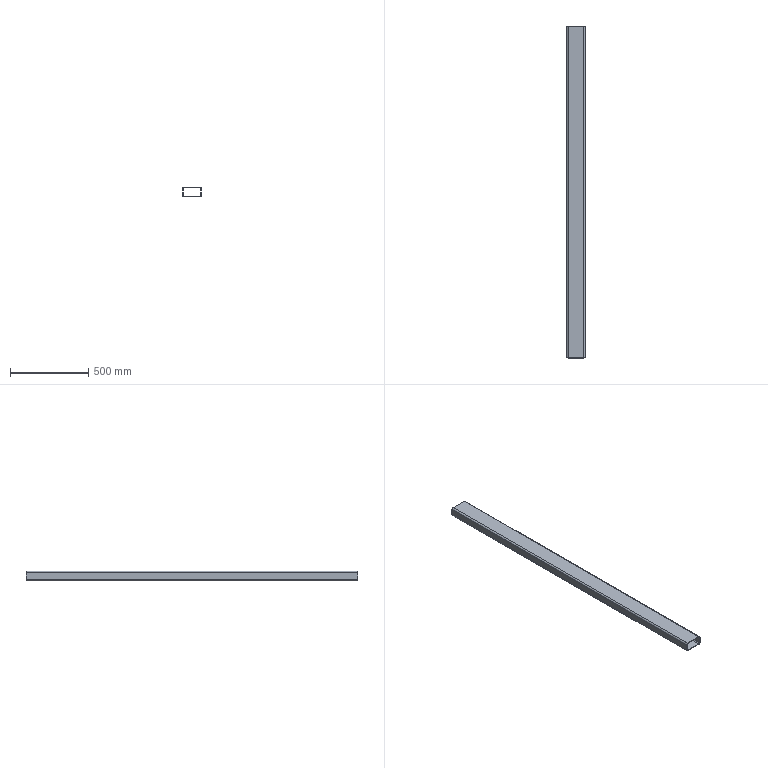Part | SolidWorks | features ExtruThin 1 | 1 solid | 18 faces | box 120 x 2124 x 60 mm | volume 2805936 mm3 | plane 10 | cylinder 8 | commonest cylinder face diameters 12 x4 20 x4
STEP:
#1=CARTESIAN_POINT('',(60.,1062.,-20.));
#2=VERTEX_POINT('',#1);
#3=CARTESIAN_POINT('',(50.,1062.,-30.));
#4=VERTEX_POINT('',#3);
#5=CARTESIAN_POINT('',(50.,1062.,-20.));
#6=DIRECTION('',(0.,1.,0.));
#7=DIRECTION('',(0.,0.,-1.));
#8=AXIS2_PLACEMENT_3D('',#5,#6,#7);
#9=CIRCLE('',#8,10.);
#10=EDGE_CURVE('',#2,#4,#9,.T.);
#11=ORIENTED_EDGE('',*,*,#10,.T.);
#12=CARTESIAN_POINT('',(-50.,1062.,-30.));
#13=VERTEX_POINT('',#12);
#14=CARTESIAN_POINT('',(-50.,1062.,-30.));
#15=DIRECTION('',(-1.,0.,0.));
#16=VECTOR('',#15,1000.);
#17=LINE('',#14,#16);
#18=EDGE_CURVE('',#4,#13,#17,.T.);
#19=ORIENTED_EDGE('',*,*,#18,.T.);
#20=CARTESIAN_POINT('',(-60.,1062.,-20.));
#21=VERTEX_POINT('',#20);
#22=CARTESIAN_POINT('',(-50.,1062.,-20.));
#23=DIRECTION('',(0.,1.,0.));
#24=DIRECTION('',(0.,0.,1.));
#25=AXIS2_PLACEMENT_3D('',#22,#23,#24);
#26=CIRCLE('',#25,10.);
#27=EDGE_CURVE('',#13,#21,#26,.T.);
#28=ORIENTED_EDGE('',*,*,#27,.T.);
#29=CARTESIAN_POINT('',(-60.,1062.,20.));
#30=VERTEX_POINT('',#29);
#31=CARTESIAN_POINT('',(-60.,1062.,-20.));
#32=DIRECTION('',(0.,0.,1.));
#33=VECTOR('',#32,1000.);
#34=LINE('',#31,#33);
#35=EDGE_CURVE('',#21,#30,#34,.T.);
#36=ORIENTED_EDGE('',*,*,#35,.T.);
#37=CARTESIAN_POINT('',(-50.,1062.,30.));
#38=VERTEX_POINT('',#37);
#39=CARTESIAN_POINT('',(-50.,1062.,20.));
#40=DIRECTION('',(0.,1.,0.));
#41=DIRECTION('',(0.,0.,1.));
#42=AXIS2_PLACEMENT_3D('',#39,#40,#41);
#43=CIRCLE('',#42,10.);
#44=EDGE_CURVE('',#30,#38,#43,.T.);
#45=ORIENTED_EDGE('',*,*,#44,.T.);
#46=CARTESIAN_POINT('',(50.,1062.,30.));
#47=VERTEX_POINT('',#46);
#48=CARTESIAN_POINT('',(-50.,1062.,30.));
#49=DIRECTION('',(1.,0.,0.));
#50=VECTOR('',#49,1000.);
#51=LINE('',#48,#50);
#52=EDGE_CURVE('',#38,#47,#51,.T.);
#53=ORIENTED_EDGE('',*,*,#52,.T.);
#54=CARTESIAN_POINT('',(60.,1062.,20.));
#55=VERTEX_POINT('',#54);
#56=CARTESIAN_POINT('',(50.,1062.,20.));
#57=DIRECTION('',(0.,1.,0.));
#58=DIRECTION('',(0.,0.,1.));
#59=AXIS2_PLACEMENT_3D('',#56,#57,#58);
#60=CIRCLE('',#59,10.);
#61=EDGE_CURVE('',#47,#55,#60,.T.);
#62=ORIENTED_EDGE('',*,*,#61,.T.);
#63=CARTESIAN_POINT('',(60.,1062.,-20.));
#64=DIRECTION('',(0.,0.,-1.));
#65=VECTOR('',#64,1000.);
#66=LINE('',#63,#65);
#67=EDGE_CURVE('',#55,#2,#66,.T.);
#68=ORIENTED_EDGE('',*,*,#67,.T.);
#69=EDGE_LOOP('',(#11,#19,#28,#36,#45,#53,#62,#68));
#70=FACE_OUTER_BOUND('',#69,.T.);
#71=CARTESIAN_POINT('',(50.,1062.,-26.));
#72=VERTEX_POINT('',#71);
#73=CARTESIAN_POINT('',(-50.,1062.,-26.));
#74=VERTEX_POINT('',#73);
#75=CARTESIAN_POINT('',(50.,1062.,-26.));
#76=DIRECTION('',(-1.,0.,0.));
#77=VECTOR('',#76,1000.);
#78=LINE('',#75,#77);
#79=EDGE_CURVE('',#72,#74,#78,.T.);
#80=ORIENTED_EDGE('',*,*,#79,.F.);
#81=CARTESIAN_POINT('',(56.,1062.,-20.));
#82=VERTEX_POINT('',#81);
#83=CARTESIAN_POINT('',(50.,1062.,-20.));
#84=DIRECTION('',(0.,1.,0.));
#85=DIRECTION('',(-1.,0.,0.));
#86=AXIS2_PLACEMENT_3D('',#83,#84,#85);
#87=CIRCLE('',#86,6.);
#88=EDGE_CURVE('',#82,#72,#87,.T.);
#89=ORIENTED_EDGE('',*,*,#88,.F.);
#90=CARTESIAN_POINT('',(56.,1062.,20.));
#91=VERTEX_POINT('',#90);
#92=CARTESIAN_POINT('',(56.,1062.,-20.));
#93=DIRECTION('',(0.,0.,-1.));
#94=VECTOR('',#93,1000.);
#95=LINE('',#92,#94);
#96=EDGE_CURVE('',#91,#82,#95,.T.);
#97=ORIENTED_EDGE('',*,*,#96,.F.);
#98=CARTESIAN_POINT('',(50.,1062.,26.));
#99=VERTEX_POINT('',#98);
#100=CARTESIAN_POINT('',(50.,1062.,20.));
#101=DIRECTION('',(0.,1.,0.));
#102=DIRECTION('',(-1.,0.,0.));
#103=AXIS2_PLACEMENT_3D('',#100,#101,#102);
#104=CIRCLE('',#103,6.);
#105=EDGE_CURVE('',#99,#91,#104,.T.);
#106=ORIENTED_EDGE('',*,*,#105,.F.);
#107=CARTESIAN_POINT('',(-50.,1062.,26.));
#108=VERTEX_POINT('',#107);
#109=CARTESIAN_POINT('',(50.,1062.,26.));
#110=DIRECTION('',(1.,0.,0.));
#111=VECTOR('',#110,1000.);
#112=LINE('',#109,#111);
#113=EDGE_CURVE('',#108,#99,#112,.T.);
#114=ORIENTED_EDGE('',*,*,#113,.F.);
#115=CARTESIAN_POINT('',(-56.,1062.,20.));
#116=VERTEX_POINT('',#115);
#117=CARTESIAN_POINT('',(-50.,1062.,20.));
#118=DIRECTION('',(0.,1.,0.));
#119=DIRECTION('',(-1.,0.,0.));
#120=AXIS2_PLACEMENT_3D('',#117,#118,#119);
#121=CIRCLE('',#120,6.);
#122=EDGE_CURVE('',#116,#108,#121,.T.);
#123=ORIENTED_EDGE('',*,*,#122,.F.);
#124=CARTESIAN_POINT('',(-56.,1062.,-20.));
#125=VERTEX_POINT('',#124);
#126=CARTESIAN_POINT('',(-56.,1062.,-20.));
#127=DIRECTION('',(0.,0.,1.));
#128=VECTOR('',#127,1000.);
#129=LINE('',#126,#128);
#130=EDGE_CURVE('',#125,#116,#129,.T.);
#131=ORIENTED_EDGE('',*,*,#130,.F.);
#132=CARTESIAN_POINT('',(-50.,1062.,-20.));
#133=DIRECTION('',(0.,1.,0.));
#134=DIRECTION('',(-1.,0.,0.));
#135=AXIS2_PLACEMENT_3D('',#132,#133,#134);
#136=CIRCLE('',#135,6.);
#137=EDGE_CURVE('',#74,#125,#136,.T.);
#138=ORIENTED_EDGE('',*,*,#137,.F.);
#139=EDGE_LOOP('',(#80,#89,#97,#106,#114,#123,#131,#138));
#140=FACE_BOUND('',#139,.T.);
#141=CARTESIAN_POINT('',(50.,1062.,-20.));
#142=DIRECTION('',(0.,1.,0.));
#143=DIRECTION('',(0.,0.,1.));
#144=AXIS2_PLACEMENT_3D('',#141,#142,#143);
#145=PLANE('',#144);
#146=ADVANCED_FACE('',(#70,#140),#145,.T.);
#147=CARTESIAN_POINT('',(60.,-1062.,-20.));
#148=VERTEX_POINT('',#147);
#149=CARTESIAN_POINT('',(50.,-1062.,-30.));
#150=VERTEX_POINT('',#149);
#151=CARTESIAN_POINT('',(50.,-1062.,-20.));
#152=DIRECTION('',(0.,1.,0.));
#153=DIRECTION('',(0.,0.,-1.));
#154=AXIS2_PLACEMENT_3D('',#151,#152,#153);
#155=CIRCLE('',#154,10.);
#156=EDGE_CURVE('',#148,#150,#155,.T.);
#157=ORIENTED_EDGE('',*,*,#156,.F.);
#158=CARTESIAN_POINT('',(60.,-1062.,20.));
#159=VERTEX_POINT('',#158);
#160=CARTESIAN_POINT('',(60.,-1062.,-20.));
#161=DIRECTION('',(0.,0.,-1.));
#162=VECTOR('',#161,1000.);
#163=LINE('',#160,#162);
#164=EDGE_CURVE('',#159,#148,#163,.T.);
#165=ORIENTED_EDGE('',*,*,#164,.F.);
#166=CARTESIAN_POINT('',(50.,-1062.,30.));
#167=VERTEX_POINT('',#166);
#168=CARTESIAN_POINT('',(50.,-1062.,20.));
#169=DIRECTION('',(0.,1.,0.));
#170=DIRECTION('',(0.,0.,1.));
#171=AXIS2_PLACEMENT_3D('',#168,#169,#170);
#172=CIRCLE('',#171,10.);
#173=EDGE_CURVE('',#167,#159,#172,.T.);
#174=ORIENTED_EDGE('',*,*,#173,.F.);
#175=CARTESIAN_POINT('',(-50.,-1062.,30.));
#176=VERTEX_POINT('',#175);
#177=CARTESIAN_POINT('',(-50.,-1062.,30.));
#178=DIRECTION('',(1.,0.,0.));
#179=VECTOR('',#178,1000.);
#180=LINE('',#177,#179);
#181=EDGE_CURVE('',#176,#167,#180,.T.);
#182=ORIENTED_EDGE('',*,*,#181,.F.);
#183=CARTESIAN_POINT('',(-60.,-1062.,20.));
#184=VERTEX_POINT('',#183);
#185=CARTESIAN_POINT('',(-50.,-1062.,20.));
#186=DIRECTION('',(0.,1.,0.));
#187=DIRECTION('',(0.,0.,1.));
#188=AXIS2_PLACEMENT_3D('',#185,#186,#187);
#189=CIRCLE('',#188,10.);
#190=EDGE_CURVE('',#184,#176,#189,.T.);
#191=ORIENTED_EDGE('',*,*,#190,.F.);
#192=CARTESIAN_POINT('',(-60.,-1062.,-20.));
#193=VERTEX_POINT('',#192);
#194=CARTESIAN_POINT('',(-60.,-1062.,-20.));
#195=DIRECTION('',(0.,0.,1.));
#196=VECTOR('',#195,1000.);
#197=LINE('',#194,#196);
#198=EDGE_CURVE('',#193,#184,#197,.T.);
#199=ORIENTED_EDGE('',*,*,#198,.F.);
#200=CARTESIAN_POINT('',(-50.,-1062.,-30.));
#201=VERTEX_POINT('',#200);
#202=CARTESIAN_POINT('',(-50.,-1062.,-20.));
#203=DIRECTION('',(0.,1.,0.));
#204=DIRECTION('',(0.,0.,1.));
#205=AXIS2_PLACEMENT_3D('',#202,#203,#204);
#206=CIRCLE('',#205,10.);
#207=EDGE_CURVE('',#201,#193,#206,.T.);
#208=ORIENTED_EDGE('',*,*,#207,.F.);
#209=CARTESIAN_POINT('',(-50.,-1062.,-30.));
#210=DIRECTION('',(-1.,0.,0.));
#211=VECTOR('',#210,1000.);
#212=LINE('',#209,#211);
#213=EDGE_CURVE('',#150,#201,#212,.T.);
#214=ORIENTED_EDGE('',*,*,#213,.F.);
#215=EDGE_LOOP('',(#157,#165,#174,#182,#191,#199,#208,#214));
#216=FACE_OUTER_BOUND('',#215,.T.);
#217=CARTESIAN_POINT('',(56.,-1062.,-20.));
#218=VERTEX_POINT('',#217);
#219=CARTESIAN_POINT('',(50.,-1062.,-26.));
#220=VERTEX_POINT('',#219);
#221=CARTESIAN_POINT('',(50.,-1062.,-20.));
#222=DIRECTION('',(0.,1.,0.));
#223=DIRECTION('',(-1.,0.,0.));
#224=AXIS2_PLACEMENT_3D('',#221,#222,#223);
#225=CIRCLE('',#224,6.);
#226=EDGE_CURVE('',#218,#220,#225,.T.);
#227=ORIENTED_EDGE('',*,*,#226,.T.);
#228=CARTESIAN_POINT('',(-50.,-1062.,-26.));
#229=VERTEX_POINT('',#228);
#230=CARTESIAN_POINT('',(50.,-1062.,-26.));
#231=DIRECTION('',(-1.,0.,0.));
#232=VECTOR('',#231,1000.);
#233=LINE('',#230,#232);
#234=EDGE_CURVE('',#220,#229,#233,.T.);
#235=ORIENTED_EDGE('',*,*,#234,.T.);
#236=CARTESIAN_POINT('',(-56.,-1062.,-20.));
#237=VERTEX_POINT('',#236);
#238=CARTESIAN_POINT('',(-50.,-1062.,-20.));
#239=DIRECTION('',(0.,1.,0.));
#240=DIRECTION('',(-1.,0.,0.));
#241=AXIS2_PLACEMENT_3D('',#238,#239,#240);
#242=CIRCLE('',#241,6.);
#243=EDGE_CURVE('',#229,#237,#242,.T.);
#244=ORIENTED_EDGE('',*,*,#243,.T.);
#245=CARTESIAN_POINT('',(-56.,-1062.,20.));
#246=VERTEX_POINT('',#245);
#247=CARTESIAN_POINT('',(-56.,-1062.,-20.));
#248=DIRECTION('',(0.,0.,1.));
#249=VECTOR('',#248,1000.);
#250=LINE('',#247,#249);
#251=EDGE_CURVE('',#237,#246,#250,.T.);
#252=ORIENTED_EDGE('',*,*,#251,.T.);
#253=CARTESIAN_POINT('',(-50.,-1062.,26.));
#254=VERTEX_POINT('',#253);
#255=CARTESIAN_POINT('',(-50.,-1062.,20.));
#256=DIRECTION('',(0.,1.,0.));
#257=DIRECTION('',(-1.,0.,0.));
#258=AXIS2_PLACEMENT_3D('',#255,#256,#257);
#259=CIRCLE('',#258,6.);
#260=EDGE_CURVE('',#246,#254,#259,.T.);
#261=ORIENTED_EDGE('',*,*,#260,.T.);
#262=CARTESIAN_POINT('',(50.,-1062.,26.));
#263=VERTEX_POINT('',#262);
#264=CARTESIAN_POINT('',(50.,-1062.,26.));
#265=DIRECTION('',(1.,0.,0.));
#266=VECTOR('',#265,1000.);
#267=LINE('',#264,#266);
#268=EDGE_CURVE('',#254,#263,#267,.T.);
#269=ORIENTED_EDGE('',*,*,#268,.T.);
#270=CARTESIAN_POINT('',(56.,-1062.,20.));
#271=VERTEX_POINT('',#270);
#272=CARTESIAN_POINT('',(50.,-1062.,20.));
#273=DIRECTION('',(0.,1.,0.));
#274=DIRECTION('',(-1.,0.,0.));
#275=AXIS2_PLACEMENT_3D('',#272,#273,#274);
#276=CIRCLE('',#275,6.);
#277=EDGE_CURVE('',#263,#271,#276,.T.);
#278=ORIENTED_EDGE('',*,*,#277,.T.);
#279=CARTESIAN_POINT('',(56.,-1062.,-20.));
#280=DIRECTION('',(0.,0.,-1.));
#281=VECTOR('',#280,1000.);
#282=LINE('',#279,#281);
#283=EDGE_CURVE('',#271,#218,#282,.T.);
#284=ORIENTED_EDGE('',*,*,#283,.T.);
#285=EDGE_LOOP('',(#227,#235,#244,#252,#261,#269,#278,#284));
#286=FACE_BOUND('',#285,.T.);
#287=CARTESIAN_POINT('',(50.,-1062.,-20.));
#288=DIRECTION('',(0.,1.,0.));
#289=DIRECTION('',(0.,0.,1.));
#290=AXIS2_PLACEMENT_3D('',#287,#288,#289);
#291=PLANE('',#290);
#292=ADVANCED_FACE('',(#216,#286),#291,.F.);
#293=ORIENTED_EDGE('',*,*,#156,.T.);
#294=CARTESIAN_POINT('',(50.,1062.,-30.));
#295=DIRECTION('',(0.,-1.,0.));
#296=VECTOR('',#295,1000.);
#297=LINE('',#294,#296);
#298=EDGE_CURVE('',#4,#150,#297,.T.);
#299=ORIENTED_EDGE('',*,*,#298,.F.);
#300=ORIENTED_EDGE('',*,*,#10,.F.);
#301=CARTESIAN_POINT('',(60.,1062.,-20.));
#302=DIRECTION('',(0.,-1.,0.));
#303=VECTOR('',#302,1000.);
#304=LINE('',#301,#303);
#305=EDGE_CURVE('',#2,#148,#304,.T.);
#306=ORIENTED_EDGE('',*,*,#305,.T.);
#307=EDGE_LOOP('',(#293,#299,#300,#306));
#308=FACE_OUTER_BOUND('',#307,.T.);
#309=CARTESIAN_POINT('',(50.,1062.,-20.));
#310=DIRECTION('',(0.,-1.,0.));
#311=DIRECTION('',(0.,0.,-1.));
#312=AXIS2_PLACEMENT_3D('',#309,#310,#311);
#313=CYLINDRICAL_SURFACE('',#312,10.);
#314=ADVANCED_FACE('',(#308),#313,.T.);
#315=ORIENTED_EDGE('',*,*,#213,.T.);
#316=CARTESIAN_POINT('',(-50.,1062.,-30.));
#317=DIRECTION('',(0.,-1.,0.));
#318=VECTOR('',#317,1000.);
#319=LINE('',#316,#318);
#320=EDGE_CURVE('',#13,#201,#319,.T.);
#321=ORIENTED_EDGE('',*,*,#320,.F.);
#322=ORIENTED_EDGE('',*,*,#18,.F.);
#323=ORIENTED_EDGE('',*,*,#298,.T.);
#324=EDGE_LOOP('',(#315,#321,#322,#323));
#325=FACE_OUTER_BOUND('',#324,.T.);
#326=CARTESIAN_POINT('',(-50.,1062.,-30.));
#327=DIRECTION('',(0.,0.,1.));
#328=DIRECTION('',(1.,0.,0.));
#329=AXIS2_PLACEMENT_3D('',#326,#327,#328);
#330=PLANE('',#329);
#331=ADVANCED_FACE('',(#325),#330,.F.);
#332=ORIENTED_EDGE('',*,*,#207,.T.);
#333=CARTESIAN_POINT('',(-60.,1062.,-20.));
#334=DIRECTION('',(0.,-1.,0.));
#335=VECTOR('',#334,1000.);
#336=LINE('',#333,#335);
#337=EDGE_CURVE('',#21,#193,#336,.T.);
#338=ORIENTED_EDGE('',*,*,#337,.F.);
#339=ORIENTED_EDGE('',*,*,#27,.F.);
#340=ORIENTED_EDGE('',*,*,#320,.T.);
#341=EDGE_LOOP('',(#332,#338,#339,#340));
#342=FACE_OUTER_BOUND('',#341,.T.);
#343=CARTESIAN_POINT('',(-50.,1062.,-20.));
#344=DIRECTION('',(0.,-1.,0.));
#345=DIRECTION('',(0.,0.,-1.));
#346=AXIS2_PLACEMENT_3D('',#343,#344,#345);
#347=CYLINDRICAL_SURFACE('',#346,10.);
#348=ADVANCED_FACE('',(#342),#347,.T.);
#349=ORIENTED_EDGE('',*,*,#198,.T.);
#350=CARTESIAN_POINT('',(-60.,1062.,20.));
#351=DIRECTION('',(0.,-1.,0.));
#352=VECTOR('',#351,1000.);
#353=LINE('',#350,#352);
#354=EDGE_CURVE('',#30,#184,#353,.T.);
#355=ORIENTED_EDGE('',*,*,#354,.F.);
#356=ORIENTED_EDGE('',*,*,#35,.F.);
#357=ORIENTED_EDGE('',*,*,#337,.T.);
#358=EDGE_LOOP('',(#349,#355,#356,#357));
#359=FACE_OUTER_BOUND('',#358,.T.);
#360=CARTESIAN_POINT('',(-60.,1062.,-20.));
#361=DIRECTION('',(1.,0.,0.));
#362=DIRECTION('',(0.,0.,-1.));
#363=AXIS2_PLACEMENT_3D('',#360,#361,#362);
#364=PLANE('',#363);
#365=ADVANCED_FACE('',(#359),#364,.F.);
#366=ORIENTED_EDGE('',*,*,#190,.T.);
#367=CARTESIAN_POINT('',(-50.,1062.,30.));
#368=DIRECTION('',(0.,-1.,0.));
#369=VECTOR('',#368,1000.);
#370=LINE('',#367,#369);
#371=EDGE_CURVE('',#38,#176,#370,.T.);
#372=ORIENTED_EDGE('',*,*,#371,.F.);
#373=ORIENTED_EDGE('',*,*,#44,.F.);
#374=ORIENTED_EDGE('',*,*,#354,.T.);
#375=EDGE_LOOP('',(#366,#372,#373,#374));
#376=FACE_OUTER_BOUND('',#375,.T.);
#377=CARTESIAN_POINT('',(-50.,1062.,20.));
#378=DIRECTION('',(0.,-1.,0.));
#379=DIRECTION('',(0.,0.,-1.));
#380=AXIS2_PLACEMENT_3D('',#377,#378,#379);
#381=CYLINDRICAL_SURFACE('',#380,10.);
#382=ADVANCED_FACE('',(#376),#381,.T.);
#383=ORIENTED_EDGE('',*,*,#181,.T.);
#384=CARTESIAN_POINT('',(50.,1062.,30.));
#385=DIRECTION('',(0.,-1.,0.));
#386=VECTOR('',#385,1000.);
#387=LINE('',#384,#386);
#388=EDGE_CURVE('',#47,#167,#387,.T.);
#389=ORIENTED_EDGE('',*,*,#388,.F.);
#390=ORIENTED_EDGE('',*,*,#52,.F.);
#391=ORIENTED_EDGE('',*,*,#371,.T.);
#392=EDGE_LOOP('',(#383,#389,#390,#391));
#393=FACE_OUTER_BOUND('',#392,.T.);
#394=CARTESIAN_POINT('',(-50.,1062.,30.));
#395=DIRECTION('',(0.,0.,-1.));
#396=DIRECTION('',(-1.,0.,0.));
#397=AXIS2_PLACEMENT_3D('',#394,#395,#396);
#398=PLANE('',#397);
#399=ADVANCED_FACE('',(#393),#398,.F.);
#400=ORIENTED_EDGE('',*,*,#173,.T.);
#401=CARTESIAN_POINT('',(60.,1062.,20.));
#402=DIRECTION('',(0.,-1.,0.));
#403=VECTOR('',#402,1000.);
#404=LINE('',#401,#403);
#405=EDGE_CURVE('',#55,#159,#404,.T.);
#406=ORIENTED_EDGE('',*,*,#405,.F.);
#407=ORIENTED_EDGE('',*,*,#61,.F.);
#408=ORIENTED_EDGE('',*,*,#388,.T.);
#409=EDGE_LOOP('',(#400,#406,#407,#408));
#410=FACE_OUTER_BOUND('',#409,.T.);
#411=CARTESIAN_POINT('',(50.,1062.,20.));
#412=DIRECTION('',(0.,-1.,0.));
#413=DIRECTION('',(0.,0.,-1.));
#414=AXIS2_PLACEMENT_3D('',#411,#412,#413);
#415=CYLINDRICAL_SURFACE('',#414,10.);
#416=ADVANCED_FACE('',(#410),#415,.T.);
#417=ORIENTED_EDGE('',*,*,#164,.T.);
#418=ORIENTED_EDGE('',*,*,#305,.F.);
#419=ORIENTED_EDGE('',*,*,#67,.F.);
#420=ORIENTED_EDGE('',*,*,#405,.T.);
#421=EDGE_LOOP('',(#417,#418,#419,#420));
#422=FACE_OUTER_BOUND('',#421,.T.);
#423=CARTESIAN_POINT('',(60.,1062.,-20.));
#424=DIRECTION('',(-1.,0.,0.));
#425=DIRECTION('',(0.,0.,1.));
#426=AXIS2_PLACEMENT_3D('',#423,#424,#425);
#427=PLANE('',#426);
#428=ADVANCED_FACE('',(#422),#427,.F.);
#429=ORIENTED_EDGE('',*,*,#226,.F.);
#430=CARTESIAN_POINT('',(56.,1062.,-20.));
#431=DIRECTION('',(0.,-1.,0.));
#432=VECTOR('',#431,1000.);
#433=LINE('',#430,#432);
#434=EDGE_CURVE('',#82,#218,#433,.T.);
#435=ORIENTED_EDGE('',*,*,#434,.F.);
#436=ORIENTED_EDGE('',*,*,#88,.T.);
#437=CARTESIAN_POINT('',(50.,1062.,-26.));
#438=DIRECTION('',(0.,-1.,0.));
#439=VECTOR('',#438,1000.);
#440=LINE('',#437,#439);
#441=EDGE_CURVE('',#72,#220,#440,.T.);
#442=ORIENTED_EDGE('',*,*,#441,.T.);
#443=EDGE_LOOP('',(#429,#435,#436,#442));
#444=FACE_OUTER_BOUND('',#443,.T.);
#445=CARTESIAN_POINT('',(50.,1062.,-20.));
#446=DIRECTION('',(0.,-1.,0.));
#447=DIRECTION('',(0.,0.,-1.));
#448=AXIS2_PLACEMENT_3D('',#445,#446,#447);
#449=CYLINDRICAL_SURFACE('',#448,6.);
#450=ADVANCED_FACE('',(#444),#449,.F.);
#451=ORIENTED_EDGE('',*,*,#234,.F.);
#452=ORIENTED_EDGE('',*,*,#441,.F.);
#453=ORIENTED_EDGE('',*,*,#79,.T.);
#454=CARTESIAN_POINT('',(-50.,1062.,-26.));
#455=DIRECTION('',(0.,-1.,0.));
#456=VECTOR('',#455,1000.);
#457=LINE('',#454,#456);
#458=EDGE_CURVE('',#74,#229,#457,.T.);
#459=ORIENTED_EDGE('',*,*,#458,.T.);
#460=EDGE_LOOP('',(#451,#452,#453,#459));
#461=FACE_OUTER_BOUND('',#460,.T.);
#462=CARTESIAN_POINT('',(50.,1062.,-26.));
#463=DIRECTION('',(0.,0.,1.));
#464=DIRECTION('',(1.,0.,0.));
#465=AXIS2_PLACEMENT_3D('',#462,#463,#464);
#466=PLANE('',#465);
#467=ADVANCED_FACE('',(#461),#466,.T.);
#468=ORIENTED_EDGE('',*,*,#243,.F.);
#469=ORIENTED_EDGE('',*,*,#458,.F.);
#470=ORIENTED_EDGE('',*,*,#137,.T.);
#471=CARTESIAN_POINT('',(-56.,1062.,-20.));
#472=DIRECTION('',(0.,-1.,0.));
#473=VECTOR('',#472,1000.);
#474=LINE('',#471,#473);
#475=EDGE_CURVE('',#125,#237,#474,.T.);
#476=ORIENTED_EDGE('',*,*,#475,.T.);
#477=EDGE_LOOP('',(#468,#469,#470,#476));
#478=FACE_OUTER_BOUND('',#477,.T.);
#479=CARTESIAN_POINT('',(-50.,1062.,-20.));
#480=DIRECTION('',(0.,-1.,0.));
#481=DIRECTION('',(0.,0.,-1.));
#482=AXIS2_PLACEMENT_3D('',#479,#480,#481);
#483=CYLINDRICAL_SURFACE('',#482,6.);
#484=ADVANCED_FACE('',(#478),#483,.F.);
#485=ORIENTED_EDGE('',*,*,#251,.F.);
#486=ORIENTED_EDGE('',*,*,#475,.F.);
#487=ORIENTED_EDGE('',*,*,#130,.T.);
#488=CARTESIAN_POINT('',(-56.,1062.,20.));
#489=DIRECTION('',(0.,-1.,0.));
#490=VECTOR('',#489,1000.);
#491=LINE('',#488,#490);
#492=EDGE_CURVE('',#116,#246,#491,.T.);
#493=ORIENTED_EDGE('',*,*,#492,.T.);
#494=EDGE_LOOP('',(#485,#486,#487,#493));
#495=FACE_OUTER_BOUND('',#494,.T.);
#496=CARTESIAN_POINT('',(-56.,1062.,-20.));
#497=DIRECTION('',(1.,0.,0.));
#498=DIRECTION('',(0.,0.,-1.));
#499=AXIS2_PLACEMENT_3D('',#496,#497,#498);
#500=PLANE('',#499);
#501=ADVANCED_FACE('',(#495),#500,.T.);
#502=ORIENTED_EDGE('',*,*,#260,.F.);
#503=ORIENTED_EDGE('',*,*,#492,.F.);
#504=ORIENTED_EDGE('',*,*,#122,.T.);
#505=CARTESIAN_POINT('',(-50.,1062.,26.));
#506=DIRECTION('',(0.,-1.,0.));
#507=VECTOR('',#506,1000.);
#508=LINE('',#505,#507);
#509=EDGE_CURVE('',#108,#254,#508,.T.);
#510=ORIENTED_EDGE('',*,*,#509,.T.);
#511=EDGE_LOOP('',(#502,#503,#504,#510));
#512=FACE_OUTER_BOUND('',#511,.T.);
#513=CARTESIAN_POINT('',(-50.,1062.,20.));
#514=DIRECTION('',(0.,-1.,0.));
#515=DIRECTION('',(0.,0.,-1.));
#516=AXIS2_PLACEMENT_3D('',#513,#514,#515);
#517=CYLINDRICAL_SURFACE('',#516,6.);
#518=ADVANCED_FACE('',(#512),#517,.F.);
#519=ORIENTED_EDGE('',*,*,#268,.F.);
#520=ORIENTED_EDGE('',*,*,#509,.F.);
#521=ORIENTED_EDGE('',*,*,#113,.T.);
#522=CARTESIAN_POINT('',(50.,1062.,26.));
#523=DIRECTION('',(0.,-1.,0.));
#524=VECTOR('',#523,1000.);
#525=LINE('',#522,#524);
#526=EDGE_CURVE('',#99,#263,#525,.T.);
#527=ORIENTED_EDGE('',*,*,#526,.T.);
#528=EDGE_LOOP('',(#519,#520,#521,#527));
#529=FACE_OUTER_BOUND('',#528,.T.);
#530=CARTESIAN_POINT('',(50.,1062.,26.));
#531=DIRECTION('',(0.,0.,-1.));
#532=DIRECTION('',(-1.,0.,0.));
#533=AXIS2_PLACEMENT_3D('',#530,#531,#532);
#534=PLANE('',#533);
#535=ADVANCED_FACE('',(#529),#534,.T.);
#536=ORIENTED_EDGE('',*,*,#277,.F.);
#537=ORIENTED_EDGE('',*,*,#526,.F.);
#538=ORIENTED_EDGE('',*,*,#105,.T.);
#539=CARTESIAN_POINT('',(56.,1062.,20.));
#540=DIRECTION('',(0.,-1.,0.));
#541=VECTOR('',#540,1000.);
#542=LINE('',#539,#541);
#543=EDGE_CURVE('',#91,#271,#542,.T.);
#544=ORIENTED_EDGE('',*,*,#543,.T.);
#545=EDGE_LOOP('',(#536,#537,#538,#544));
#546=FACE_OUTER_BOUND('',#545,.T.);
#547=CARTESIAN_POINT('',(50.,1062.,20.));
#548=DIRECTION('',(0.,-1.,0.));
#549=DIRECTION('',(0.,0.,-1.));
#550=AXIS2_PLACEMENT_3D('',#547,#548,#549);
#551=CYLINDRICAL_SURFACE('',#550,6.);
#552=ADVANCED_FACE('',(#546),#551,.F.);
#553=ORIENTED_EDGE('',*,*,#283,.F.);
#554=ORIENTED_EDGE('',*,*,#543,.F.);
#555=ORIENTED_EDGE('',*,*,#96,.T.);
#556=ORIENTED_EDGE('',*,*,#434,.T.);
#557=EDGE_LOOP('',(#553,#554,#555,#556));
#558=FACE_OUTER_BOUND('',#557,.T.);
#559=CARTESIAN_POINT('',(56.,1062.,-20.));
#560=DIRECTION('',(-1.,0.,0.));
#561=DIRECTION('',(0.,0.,1.));
#562=AXIS2_PLACEMENT_3D('',#559,#560,#561);
#563=PLANE('',#562);
#564=ADVANCED_FACE('',(#558),#563,.T.);
#565=CLOSED_SHELL('',(#146,#292,#314,#331,#348,#365,#382,#399,#416,#428,#450,#467,#484,#501,#518,#535,#552,#564));
#566=MANIFOLD_SOLID_BREP('',#565);
#567=CARTESIAN_POINT('',(0.,0.,0.));
#568=DIRECTION('',(0.,0.,1.));
#569=DIRECTION('',(1.,0.,0.));
#570=AXIS2_PLACEMENT_3D('',#567,#568,#569);
#571=(LENGTH_UNIT()NAMED_UNIT(*)SI_UNIT(.MILLI.,.METRE.));
#572=UNCERTAINTY_MEASURE_WITH_UNIT(LENGTH_MEASURE(0.00001),#571,'','');
#573=(NAMED_UNIT(*)PLANE_ANGLE_UNIT()SI_UNIT($,.RADIAN.));
#574=(NAMED_UNIT(*)SI_UNIT($,.STERADIAN.)SOLID_ANGLE_UNIT());
#575=(GEOMETRIC_REPRESENTATION_CONTEXT(3)GLOBAL_UNCERTAINTY_ASSIGNED_CONTEXT((#572))GLOBAL_UNIT_ASSIGNED_CONTEXT((#571,#573,#574))REPRESENTATION_CONTEXT('',''));
#576=ADVANCED_BREP_SHAPE_REPRESENTATION('',(#566,#570),#575);